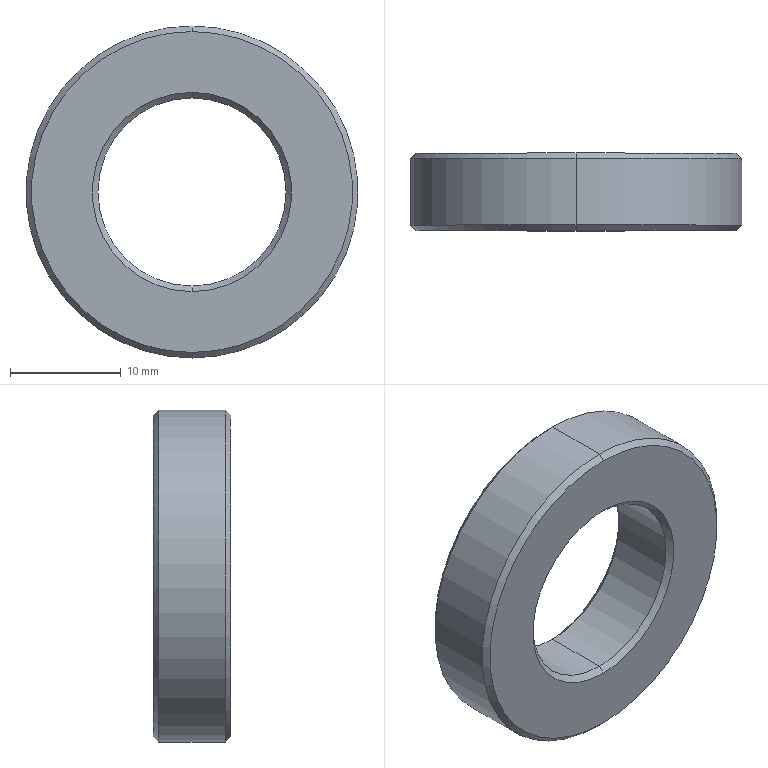Part | STEP file | 6903 ZZ | 1 solid | 14 faces | box 30 x 7 x 30 mm | volume 3322 mm3 | cone 8 | cylinder 4 | plane 2 | commonest cylinder face diameters 17 x2 30 x2
STEP:
#1=CARTESIAN_POINT('',(0.,0.,0.));
#2=DIRECTION('',(0.,0.,1.));
#3=DIRECTION('',(1.,0.,0.));
#4=AXIS2_PLACEMENT_3D('',#1,#2,#3);
#5=CARTESIAN_POINT('',(0.,6.5,8.5));
#6=VERTEX_POINT('',#5);
#7=CARTESIAN_POINT('',(0.,7.,9.));
#8=VERTEX_POINT('',#7);
#9=CARTESIAN_POINT('',(0.,6.5,8.5));
#10=DIRECTION('',(0.,0.7071,0.7071));
#11=VECTOR('',#10,1.);
#12=LINE('',#9,#11);
#13=CARTESIAN_POINT('',(0.,6.5,0.));
#14=DIRECTION('',(0.,1.,0.));
#15=DIRECTION('',(0.,0.,1.));
#16=AXIS2_PLACEMENT_3D('',#13,#14,#15);
#17=CONICAL_SURFACE('',#16,8.5,0.7854);
#18=CARTESIAN_POINT('',(6.283,0.));
#19=DIRECTION('',(0.,1.));
#20=VECTOR('',#19,1.);
#21=LINE('',#18,#20);
#22=(GEOMETRIC_REPRESENTATION_CONTEXT(2)PARAMETRIC_REPRESENTATION_CONTEXT()REPRESENTATION_CONTEXT('',''));
#23=DEFINITIONAL_REPRESENTATION('',(#21),#22);
#24=PCURVE('',#17,#23);
#25=CARTESIAN_POINT('',(0.,6.5,0.));
#26=DIRECTION('',(0.,1.,0.));
#27=DIRECTION('',(0.,0.,1.));
#28=AXIS2_PLACEMENT_3D('',#25,#26,#27);
#29=CONICAL_SURFACE('',#28,8.5,0.7854);
#30=CARTESIAN_POINT('',(0.,0.));
#31=DIRECTION('',(0.,1.));
#32=VECTOR('',#31,1.);
#33=LINE('',#30,#32);
#34=(GEOMETRIC_REPRESENTATION_CONTEXT(2)PARAMETRIC_REPRESENTATION_CONTEXT()REPRESENTATION_CONTEXT('',''));
#35=DEFINITIONAL_REPRESENTATION('',(#33),#34);
#36=PCURVE('',#29,#35);
#37=SURFACE_CURVE('',#12,(#24,#36),.PCURVE_S1.);
#38=EDGE_CURVE('',#6,#8,#37,.T.);
#39=ORIENTED_EDGE('',*,*,#38,.T.);
#40=CARTESIAN_POINT('',(0.,7.,-9.));
#41=VERTEX_POINT('',#40);
#42=CARTESIAN_POINT('',(0.,7.,0.));
#43=DIRECTION('',(0.,-1.,0.));
#44=DIRECTION('',(0.,0.,1.));
#45=AXIS2_PLACEMENT_3D('',#42,#43,#44);
#46=CIRCLE('',#45,9.);
#47=CARTESIAN_POINT('',(6.283,0.5));
#48=DIRECTION('',(-1.,0.));
#49=VECTOR('',#48,1.);
#50=LINE('',#47,#49);
#51=(GEOMETRIC_REPRESENTATION_CONTEXT(2)PARAMETRIC_REPRESENTATION_CONTEXT()REPRESENTATION_CONTEXT('',''));
#52=DEFINITIONAL_REPRESENTATION('',(#50),#51);
#53=PCURVE('',#17,#52);
#54=CARTESIAN_POINT('',(0.,7.,0.));
#55=DIRECTION('',(0.,1.,0.));
#56=DIRECTION('',(0.,0.,1.));
#57=AXIS2_PLACEMENT_3D('',#54,#55,#56);
#58=PLANE('',#57);
#59=CARTESIAN_POINT('',(9.,0.));
#60=CARTESIAN_POINT('',(9.,-15.588));
#61=CARTESIAN_POINT('',(-4.5,-7.794));
#62=CARTESIAN_POINT('',(-18.,0.));
#63=CARTESIAN_POINT('',(-4.5,7.794));
#64=CARTESIAN_POINT('',(9.,15.588));
#65=CARTESIAN_POINT('',(9.,0.));
#66=(BOUNDED_CURVE()B_SPLINE_CURVE(2,(#59,#60,#61,#62,#63,#64,#65),.UNSPECIFIED.,.T.,.F.)B_SPLINE_CURVE_WITH_KNOTS((1,2,2,2,2,1),(-2.094,0.,2.094,4.189,6.283,8.378),.UNSPECIFIED.)CURVE()GEOMETRIC_REPRESENTATION_ITEM()RATIONAL_B_SPLINE_CURVE((1.,0.5,1.,0.5,1.,0.5,1.))REPRESENTATION_ITEM(''));
#67=(GEOMETRIC_REPRESENTATION_CONTEXT(2)PARAMETRIC_REPRESENTATION_CONTEXT()REPRESENTATION_CONTEXT('',''));
#68=DEFINITIONAL_REPRESENTATION('',(#66),#67);
#69=PCURVE('',#58,#68);
#70=SURFACE_CURVE('',#46,(#53,#69),.PCURVE_S1.);
#71=EDGE_CURVE('',#8,#41,#70,.T.);
#72=ORIENTED_EDGE('',*,*,#71,.T.);
#73=CARTESIAN_POINT('',(0.,6.5,-8.5));
#74=VERTEX_POINT('',#73);
#75=CARTESIAN_POINT('',(0.,6.5,-8.5));
#76=DIRECTION('',(0.,0.7071,-0.7071));
#77=VECTOR('',#76,1.);
#78=LINE('',#75,#77);
#79=CARTESIAN_POINT('',(3.142,0.));
#80=DIRECTION('',(0.,1.));
#81=VECTOR('',#80,1.);
#82=LINE('',#79,#81);
#83=(GEOMETRIC_REPRESENTATION_CONTEXT(2)PARAMETRIC_REPRESENTATION_CONTEXT()REPRESENTATION_CONTEXT('',''));
#84=DEFINITIONAL_REPRESENTATION('',(#82),#83);
#85=PCURVE('',#17,#84);
#86=CARTESIAN_POINT('',(3.142,0.));
#87=DIRECTION('',(0.,1.));
#88=VECTOR('',#87,1.);
#89=LINE('',#86,#88);
#90=(GEOMETRIC_REPRESENTATION_CONTEXT(2)PARAMETRIC_REPRESENTATION_CONTEXT()REPRESENTATION_CONTEXT('',''));
#91=DEFINITIONAL_REPRESENTATION('',(#89),#90);
#92=PCURVE('',#29,#91);
#93=SURFACE_CURVE('',#78,(#85,#92),.PCURVE_S1.);
#94=EDGE_CURVE('',#74,#41,#93,.T.);
#95=ORIENTED_EDGE('',*,*,#94,.F.);
#96=CARTESIAN_POINT('',(0.,6.5,0.));
#97=DIRECTION('',(0.,1.,0.));
#98=DIRECTION('',(0.,0.,1.));
#99=AXIS2_PLACEMENT_3D('',#96,#97,#98);
#100=CIRCLE('',#99,8.5);
#101=CARTESIAN_POINT('',(0.,0.));
#102=DIRECTION('',(1.,0.));
#103=VECTOR('',#102,1.);
#104=LINE('',#101,#103);
#105=(GEOMETRIC_REPRESENTATION_CONTEXT(2)PARAMETRIC_REPRESENTATION_CONTEXT()REPRESENTATION_CONTEXT('',''));
#106=DEFINITIONAL_REPRESENTATION('',(#104),#105);
#107=PCURVE('',#17,#106);
#108=CARTESIAN_POINT('',(0.,7.,0.));
#109=DIRECTION('',(0.,-1.,0.));
#110=DIRECTION('',(0.,0.,-1.));
#111=AXIS2_PLACEMENT_3D('',#108,#109,#110);
#112=CYLINDRICAL_SURFACE('',#111,8.5);
#113=CARTESIAN_POINT('',(9.425,0.5));
#114=DIRECTION('',(-1.,0.));
#115=VECTOR('',#114,1.);
#116=LINE('',#113,#115);
#117=(GEOMETRIC_REPRESENTATION_CONTEXT(2)PARAMETRIC_REPRESENTATION_CONTEXT()REPRESENTATION_CONTEXT('',''));
#118=DEFINITIONAL_REPRESENTATION('',(#116),#117);
#119=PCURVE('',#112,#118);
#120=SURFACE_CURVE('',#100,(#107,#119),.PCURVE_S1.);
#121=EDGE_CURVE('',#74,#6,#120,.T.);
#122=ORIENTED_EDGE('',*,*,#121,.T.);
#123=EDGE_LOOP('',(#39,#72,#95,#122));
#124=FACE_BOUND('',#123,.F.);
#125=ADVANCED_FACE('',(#124),#17,.F.);
#126=CARTESIAN_POINT('',(0.,7.,14.5));
#127=VERTEX_POINT('',#126);
#128=CARTESIAN_POINT('',(0.,7.,-14.5));
#129=VERTEX_POINT('',#128);
#130=CARTESIAN_POINT('',(0.,7.,0.));
#131=DIRECTION('',(0.,1.,0.));
#132=DIRECTION('',(0.,0.,1.));
#133=AXIS2_PLACEMENT_3D('',#130,#131,#132);
#134=CIRCLE('',#133,14.5);
#135=CARTESIAN_POINT('',(0.,7.,0.));
#136=DIRECTION('',(0.,-1.,0.));
#137=DIRECTION('',(0.,0.,-1.));
#138=AXIS2_PLACEMENT_3D('',#135,#136,#137);
#139=CONICAL_SURFACE('',#138,14.5,0.7854);
#140=CARTESIAN_POINT('',(3.142,0.));
#141=DIRECTION('',(-1.,0.));
#142=VECTOR('',#141,1.);
#143=LINE('',#140,#142);
#144=(GEOMETRIC_REPRESENTATION_CONTEXT(2)PARAMETRIC_REPRESENTATION_CONTEXT()REPRESENTATION_CONTEXT('',''));
#145=DEFINITIONAL_REPRESENTATION('',(#143),#144);
#146=PCURVE('',#139,#145);
#147=CARTESIAN_POINT('',(0.,0.));
#148=DIRECTION('',(1.,0.));
#149=AXIS2_PLACEMENT_2D('',#147,#148);
#150=CIRCLE('',#149,14.5);
#151=(GEOMETRIC_REPRESENTATION_CONTEXT(2)PARAMETRIC_REPRESENTATION_CONTEXT()REPRESENTATION_CONTEXT('',''));
#152=DEFINITIONAL_REPRESENTATION('',(#150),#151);
#153=PCURVE('',#58,#152);
#154=SURFACE_CURVE('',#134,(#146,#153),.PCURVE_S1.);
#155=EDGE_CURVE('',#127,#129,#154,.T.);
#156=ORIENTED_EDGE('',*,*,#155,.F.);
#157=CARTESIAN_POINT('',(0.,6.5,15.));
#158=VERTEX_POINT('',#157);
#159=CARTESIAN_POINT('',(0.,7.,14.5));
#160=DIRECTION('',(0.,-0.7071,0.7071));
#161=VECTOR('',#160,1.);
#162=LINE('',#159,#161);
#163=CARTESIAN_POINT('',(3.142,0.));
#164=DIRECTION('',(0.,1.));
#165=VECTOR('',#164,1.);
#166=LINE('',#163,#165);
#167=(GEOMETRIC_REPRESENTATION_CONTEXT(2)PARAMETRIC_REPRESENTATION_CONTEXT()REPRESENTATION_CONTEXT('',''));
#168=DEFINITIONAL_REPRESENTATION('',(#166),#167);
#169=PCURVE('',#139,#168);
#170=CARTESIAN_POINT('',(0.,7.,0.));
#171=DIRECTION('',(0.,-1.,0.));
#172=DIRECTION('',(0.,0.,-1.));
#173=AXIS2_PLACEMENT_3D('',#170,#171,#172);
#174=CONICAL_SURFACE('',#173,14.5,0.7854);
#175=CARTESIAN_POINT('',(3.142,0.));
#176=DIRECTION('',(0.,1.));
#177=VECTOR('',#176,1.);
#178=LINE('',#175,#177);
#179=(GEOMETRIC_REPRESENTATION_CONTEXT(2)PARAMETRIC_REPRESENTATION_CONTEXT()REPRESENTATION_CONTEXT('',''));
#180=DEFINITIONAL_REPRESENTATION('',(#178),#179);
#181=PCURVE('',#174,#180);
#182=SURFACE_CURVE('',#162,(#169,#181),.PCURVE_S1.);
#183=EDGE_CURVE('',#127,#158,#182,.T.);
#184=ORIENTED_EDGE('',*,*,#183,.T.);
#185=CARTESIAN_POINT('',(0.,6.5,-15.));
#186=VERTEX_POINT('',#185);
#187=CARTESIAN_POINT('',(0.,6.5,0.));
#188=DIRECTION('',(0.,-1.,0.));
#189=DIRECTION('',(0.,0.,1.));
#190=AXIS2_PLACEMENT_3D('',#187,#188,#189);
#191=CIRCLE('',#190,15.);
#192=CARTESIAN_POINT('',(-3.142,0.5));
#193=DIRECTION('',(1.,0.));
#194=VECTOR('',#193,1.);
#195=LINE('',#192,#194);
#196=(GEOMETRIC_REPRESENTATION_CONTEXT(2)PARAMETRIC_REPRESENTATION_CONTEXT()REPRESENTATION_CONTEXT('',''));
#197=DEFINITIONAL_REPRESENTATION('',(#195),#196);
#198=PCURVE('',#139,#197);
#199=CARTESIAN_POINT('',(0.,7.,0.));
#200=DIRECTION('',(0.,-1.,0.));
#201=DIRECTION('',(0.,0.,-1.));
#202=AXIS2_PLACEMENT_3D('',#199,#200,#201);
#203=CYLINDRICAL_SURFACE('',#202,15.);
#204=CARTESIAN_POINT('',(-3.142,0.5));
#205=DIRECTION('',(1.,0.));
#206=VECTOR('',#205,1.);
#207=LINE('',#204,#206);
#208=(GEOMETRIC_REPRESENTATION_CONTEXT(2)PARAMETRIC_REPRESENTATION_CONTEXT()REPRESENTATION_CONTEXT('',''));
#209=DEFINITIONAL_REPRESENTATION('',(#207),#208);
#210=PCURVE('',#203,#209);
#211=SURFACE_CURVE('',#191,(#198,#210),.PCURVE_S1.);
#212=EDGE_CURVE('',#186,#158,#211,.T.);
#213=ORIENTED_EDGE('',*,*,#212,.F.);
#214=CARTESIAN_POINT('',(0.,7.,-14.5));
#215=DIRECTION('',(0.,-0.7071,-0.7071));
#216=VECTOR('',#215,1.);
#217=LINE('',#214,#216);
#218=CARTESIAN_POINT('',(0.,0.));
#219=DIRECTION('',(0.,1.));
#220=VECTOR('',#219,1.);
#221=LINE('',#218,#220);
#222=(GEOMETRIC_REPRESENTATION_CONTEXT(2)PARAMETRIC_REPRESENTATION_CONTEXT()REPRESENTATION_CONTEXT('',''));
#223=DEFINITIONAL_REPRESENTATION('',(#221),#222);
#224=PCURVE('',#139,#223);
#225=CARTESIAN_POINT('',(6.283,0.));
#226=DIRECTION('',(0.,1.));
#227=VECTOR('',#226,1.);
#228=LINE('',#225,#227);
#229=(GEOMETRIC_REPRESENTATION_CONTEXT(2)PARAMETRIC_REPRESENTATION_CONTEXT()REPRESENTATION_CONTEXT('',''));
#230=DEFINITIONAL_REPRESENTATION('',(#228),#229);
#231=PCURVE('',#174,#230);
#232=SURFACE_CURVE('',#217,(#224,#231),.PCURVE_S1.);
#233=EDGE_CURVE('',#129,#186,#232,.T.);
#234=ORIENTED_EDGE('',*,*,#233,.F.);
#235=EDGE_LOOP('',(#156,#184,#213,#234));
#236=FACE_BOUND('',#235,.T.);
#237=ADVANCED_FACE('',(#236),#139,.T.);
#238=CARTESIAN_POINT('',(0.,0.5,-8.5));
#239=VERTEX_POINT('',#238);
#240=CARTESIAN_POINT('',(0.,0.,-9.));
#241=VERTEX_POINT('',#240);
#242=CARTESIAN_POINT('',(0.,0.,-9.));
#243=DIRECTION('',(0.,-0.7071,-0.7071));
#244=VECTOR('',#243,1.);
#245=LINE('',#242,#244);
#246=CARTESIAN_POINT('',(0.,0.,0.));
#247=DIRECTION('',(0.,-1.,0.));
#248=DIRECTION('',(0.,0.,-1.));
#249=AXIS2_PLACEMENT_3D('',#246,#247,#248);
#250=CONICAL_SURFACE('',#249,9.,0.7854);
#251=CARTESIAN_POINT('',(6.283,0.));
#252=DIRECTION('',(0.,1.));
#253=VECTOR('',#252,1.);
#254=LINE('',#251,#253);
#255=(GEOMETRIC_REPRESENTATION_CONTEXT(2)PARAMETRIC_REPRESENTATION_CONTEXT()REPRESENTATION_CONTEXT('',''));
#256=DEFINITIONAL_REPRESENTATION('',(#254),#255);
#257=PCURVE('',#250,#256);
#258=CARTESIAN_POINT('',(0.,0.,0.));
#259=DIRECTION('',(0.,-1.,0.));
#260=DIRECTION('',(0.,0.,-1.));
#261=AXIS2_PLACEMENT_3D('',#258,#259,#260);
#262=CONICAL_SURFACE('',#261,9.,0.7854);
#263=CARTESIAN_POINT('',(0.,0.));
#264=DIRECTION('',(0.,1.));
#265=VECTOR('',#264,1.);
#266=LINE('',#263,#265);
#267=(GEOMETRIC_REPRESENTATION_CONTEXT(2)PARAMETRIC_REPRESENTATION_CONTEXT()REPRESENTATION_CONTEXT('',''));
#268=DEFINITIONAL_REPRESENTATION('',(#266),#267);
#269=PCURVE('',#262,#268);
#270=SURFACE_CURVE('',#245,(#257,#269),.PCURVE_S1.);
#271=EDGE_CURVE('',#239,#241,#270,.T.);
#272=ORIENTED_EDGE('',*,*,#271,.T.);
#273=CARTESIAN_POINT('',(0.,0.,9.));
#274=VERTEX_POINT('',#273);
#275=CARTESIAN_POINT('',(0.,0.,0.));
#276=DIRECTION('',(0.,1.,0.));
#277=DIRECTION('',(0.,0.,1.));
#278=AXIS2_PLACEMENT_3D('',#275,#276,#277);
#279=CIRCLE('',#278,9.);
#280=CARTESIAN_POINT('',(9.425,0.));
#281=DIRECTION('',(-1.,0.));
#282=VECTOR('',#281,1.);
#283=LINE('',#280,#282);
#284=(GEOMETRIC_REPRESENTATION_CONTEXT(2)PARAMETRIC_REPRESENTATION_CONTEXT()REPRESENTATION_CONTEXT('',''));
#285=DEFINITIONAL_REPRESENTATION('',(#283),#284);
#286=PCURVE('',#250,#285);
#287=CARTESIAN_POINT('',(0.,0.,0.));
#288=DIRECTION('',(0.,1.,0.));
#289=DIRECTION('',(0.,0.,1.));
#290=AXIS2_PLACEMENT_3D('',#287,#288,#289);
#291=PLANE('',#290);
#292=CARTESIAN_POINT('',(0.,0.));
#293=DIRECTION('',(1.,0.));
#294=AXIS2_PLACEMENT_2D('',#292,#293);
#295=CIRCLE('',#294,9.);
#296=(GEOMETRIC_REPRESENTATION_CONTEXT(2)PARAMETRIC_REPRESENTATION_CONTEXT()REPRESENTATION_CONTEXT('',''));
#297=DEFINITIONAL_REPRESENTATION('',(#295),#296);
#298=PCURVE('',#291,#297);
#299=SURFACE_CURVE('',#279,(#286,#298),.PCURVE_S1.);
#300=EDGE_CURVE('',#241,#274,#299,.T.);
#301=ORIENTED_EDGE('',*,*,#300,.T.);
#302=CARTESIAN_POINT('',(0.,0.5,8.5));
#303=VERTEX_POINT('',#302);
#304=CARTESIAN_POINT('',(0.,0.,9.));
#305=DIRECTION('',(0.,-0.7071,0.7071));
#306=VECTOR('',#305,1.);
#307=LINE('',#304,#306);
#308=CARTESIAN_POINT('',(3.142,0.));
#309=DIRECTION('',(0.,1.));
#310=VECTOR('',#309,1.);
#311=LINE('',#308,#310);
#312=(GEOMETRIC_REPRESENTATION_CONTEXT(2)PARAMETRIC_REPRESENTATION_CONTEXT()REPRESENTATION_CONTEXT('',''));
#313=DEFINITIONAL_REPRESENTATION('',(#311),#312);
#314=PCURVE('',#250,#313);
#315=CARTESIAN_POINT('',(3.142,0.));
#316=DIRECTION('',(0.,1.));
#317=VECTOR('',#316,1.);
#318=LINE('',#315,#317);
#319=(GEOMETRIC_REPRESENTATION_CONTEXT(2)PARAMETRIC_REPRESENTATION_CONTEXT()REPRESENTATION_CONTEXT('',''));
#320=DEFINITIONAL_REPRESENTATION('',(#318),#319);
#321=PCURVE('',#262,#320);
#322=SURFACE_CURVE('',#307,(#314,#321),.PCURVE_S1.);
#323=EDGE_CURVE('',#303,#274,#322,.T.);
#324=ORIENTED_EDGE('',*,*,#323,.F.);
#325=CARTESIAN_POINT('',(0.,0.5,0.));
#326=DIRECTION('',(0.,-1.,0.));
#327=DIRECTION('',(0.,0.,1.));
#328=AXIS2_PLACEMENT_3D('',#325,#326,#327);
#329=CIRCLE('',#328,8.5);
#330=CARTESIAN_POINT('',(3.142,-0.5));
#331=DIRECTION('',(1.,0.));
#332=VECTOR('',#331,1.);
#333=LINE('',#330,#332);
#334=(GEOMETRIC_REPRESENTATION_CONTEXT(2)PARAMETRIC_REPRESENTATION_CONTEXT()REPRESENTATION_CONTEXT('',''));
#335=DEFINITIONAL_REPRESENTATION('',(#333),#334);
#336=PCURVE('',#250,#335);
#337=CARTESIAN_POINT('',(3.142,6.5));
#338=DIRECTION('',(1.,0.));
#339=VECTOR('',#338,1.);
#340=LINE('',#337,#339);
#341=(GEOMETRIC_REPRESENTATION_CONTEXT(2)PARAMETRIC_REPRESENTATION_CONTEXT()REPRESENTATION_CONTEXT('',''));
#342=DEFINITIONAL_REPRESENTATION('',(#340),#341);
#343=PCURVE('',#112,#342);
#344=SURFACE_CURVE('',#329,(#336,#343),.PCURVE_S1.);
#345=EDGE_CURVE('',#303,#239,#344,.T.);
#346=ORIENTED_EDGE('',*,*,#345,.T.);
#347=EDGE_LOOP('',(#272,#301,#324,#346));
#348=FACE_BOUND('',#347,.F.);
#349=ADVANCED_FACE('',(#348),#250,.F.);
#350=CARTESIAN_POINT('',(0.,0.,-14.5));
#351=VERTEX_POINT('',#350);
#352=CARTESIAN_POINT('',(0.,0.,14.5));
#353=VERTEX_POINT('',#352);
#354=CARTESIAN_POINT('',(0.,0.,0.));
#355=DIRECTION('',(0.,-1.,0.));
#356=DIRECTION('',(0.,0.,1.));
#357=AXIS2_PLACEMENT_3D('',#354,#355,#356);
#358=CIRCLE('',#357,14.5);
#359=CARTESIAN_POINT('',(0.,0.5,0.));
#360=DIRECTION('',(0.,1.,0.));
#361=DIRECTION('',(0.,0.,1.));
#362=AXIS2_PLACEMENT_3D('',#359,#360,#361);
#363=CONICAL_SURFACE('',#362,15.,0.7854);
#364=CARTESIAN_POINT('',(6.283,-0.5));
#365=DIRECTION('',(-1.,0.));
#366=VECTOR('',#365,1.);
#367=LINE('',#364,#366);
#368=(GEOMETRIC_REPRESENTATION_CONTEXT(2)PARAMETRIC_REPRESENTATION_CONTEXT()REPRESENTATION_CONTEXT('',''));
#369=DEFINITIONAL_REPRESENTATION('',(#367),#368);
#370=PCURVE('',#363,#369);
#371=CARTESIAN_POINT('',(14.5,0.));
#372=CARTESIAN_POINT('',(14.5,-25.115));
#373=CARTESIAN_POINT('',(-7.25,-12.557));
#374=CARTESIAN_POINT('',(-29.,0.));
#375=CARTESIAN_POINT('',(-7.25,12.557));
#376=CARTESIAN_POINT('',(14.5,25.115));
#377=CARTESIAN_POINT('',(14.5,0.));
#378=(BOUNDED_CURVE()B_SPLINE_CURVE(2,(#371,#372,#373,#374,#375,#376,#377),.UNSPECIFIED.,.T.,.F.)B_SPLINE_CURVE_WITH_KNOTS((1,2,2,2,2,1),(-2.094,0.,2.094,4.189,6.283,8.378),.UNSPECIFIED.)CURVE()GEOMETRIC_REPRESENTATION_ITEM()RATIONAL_B_SPLINE_CURVE((1.,0.5,1.,0.5,1.,0.5,1.))REPRESENTATION_ITEM(''));
#379=(GEOMETRIC_REPRESENTATION_CONTEXT(2)PARAMETRIC_REPRESENTATION_CONTEXT()REPRESENTATION_CONTEXT('',''));
#380=DEFINITIONAL_REPRESENTATION('',(#378),#379);
#381=PCURVE('',#291,#380);
#382=SURFACE_CURVE('',#358,(#370,#381),.PCURVE_S1.);
#383=EDGE_CURVE('',#351,#353,#382,.T.);
#384=ORIENTED_EDGE('',*,*,#383,.F.);
#385=CARTESIAN_POINT('',(0.,0.5,-15.));
#386=VERTEX_POINT('',#385);
#387=CARTESIAN_POINT('',(0.,0.5,-15.));
#388=DIRECTION('',(0.,0.7071,-0.7071));
#389=VECTOR('',#388,1.);
#390=LINE('',#387,#389);
#391=CARTESIAN_POINT('',(3.142,0.));
#392=DIRECTION('',(0.,1.));
#393=VECTOR('',#392,1.);
#394=LINE('',#391,#393);
#395=(GEOMETRIC_REPRESENTATION_CONTEXT(2)PARAMETRIC_REPRESENTATION_CONTEXT()REPRESENTATION_CONTEXT('',''));
#396=DEFINITIONAL_REPRESENTATION('',(#394),#395);
#397=PCURVE('',#363,#396);
#398=CARTESIAN_POINT('',(0.,0.5,0.));
#399=DIRECTION('',(0.,1.,0.));
#400=DIRECTION('',(0.,0.,1.));
#401=AXIS2_PLACEMENT_3D('',#398,#399,#400);
#402=CONICAL_SURFACE('',#401,15.,0.7854);
#403=CARTESIAN_POINT('',(3.142,0.));
#404=DIRECTION('',(0.,1.));
#405=VECTOR('',#404,1.);
#406=LINE('',#403,#405);
#407=(GEOMETRIC_REPRESENTATION_CONTEXT(2)PARAMETRIC_REPRESENTATION_CONTEXT()REPRESENTATION_CONTEXT('',''));
#408=DEFINITIONAL_REPRESENTATION('',(#406),#407);
#409=PCURVE('',#402,#408);
#410=SURFACE_CURVE('',#390,(#397,#409),.PCURVE_S1.);
#411=EDGE_CURVE('',#351,#386,#410,.T.);
#412=ORIENTED_EDGE('',*,*,#411,.T.);
#413=CARTESIAN_POINT('',(0.,0.5,15.));
#414=VERTEX_POINT('',#413);
#415=CARTESIAN_POINT('',(0.,0.5,0.));
#416=DIRECTION('',(0.,1.,0.));
#417=DIRECTION('',(0.,0.,1.));
#418=AXIS2_PLACEMENT_3D('',#415,#416,#417);
#419=CIRCLE('',#418,15.);
#420=CARTESIAN_POINT('',(0.,0.));
#421=DIRECTION('',(1.,0.));
#422=VECTOR('',#421,1.);
#423=LINE('',#420,#422);
#424=(GEOMETRIC_REPRESENTATION_CONTEXT(2)PARAMETRIC_REPRESENTATION_CONTEXT()REPRESENTATION_CONTEXT('',''));
#425=DEFINITIONAL_REPRESENTATION('',(#423),#424);
#426=PCURVE('',#363,#425);
#427=CARTESIAN_POINT('',(3.142,6.5));
#428=DIRECTION('',(-1.,0.));
#429=VECTOR('',#428,1.);
#430=LINE('',#427,#429);
#431=(GEOMETRIC_REPRESENTATION_CONTEXT(2)PARAMETRIC_REPRESENTATION_CONTEXT()REPRESENTATION_CONTEXT('',''));
#432=DEFINITIONAL_REPRESENTATION('',(#430),#431);
#433=PCURVE('',#203,#432);
#434=SURFACE_CURVE('',#419,(#426,#433),.PCURVE_S1.);
#435=EDGE_CURVE('',#414,#386,#434,.T.);
#436=ORIENTED_EDGE('',*,*,#435,.F.);
#437=CARTESIAN_POINT('',(0.,0.5,15.));
#438=DIRECTION('',(0.,0.7071,0.7071));
#439=VECTOR('',#438,1.);
#440=LINE('',#437,#439);
#441=CARTESIAN_POINT('',(0.,0.));
#442=DIRECTION('',(0.,1.));
#443=VECTOR('',#442,1.);
#444=LINE('',#441,#443);
#445=(GEOMETRIC_REPRESENTATION_CONTEXT(2)PARAMETRIC_REPRESENTATION_CONTEXT()REPRESENTATION_CONTEXT('',''));
#446=DEFINITIONAL_REPRESENTATION('',(#444),#445);
#447=PCURVE('',#363,#446);
#448=CARTESIAN_POINT('',(6.283,0.));
#449=DIRECTION('',(0.,1.));
#450=VECTOR('',#449,1.);
#451=LINE('',#448,#450);
#452=(GEOMETRIC_REPRESENTATION_CONTEXT(2)PARAMETRIC_REPRESENTATION_CONTEXT()REPRESENTATION_CONTEXT('',''));
#453=DEFINITIONAL_REPRESENTATION('',(#451),#452);
#454=PCURVE('',#402,#453);
#455=SURFACE_CURVE('',#440,(#447,#454),.PCURVE_S1.);
#456=EDGE_CURVE('',#353,#414,#455,.T.);
#457=ORIENTED_EDGE('',*,*,#456,.F.);
#458=EDGE_LOOP('',(#384,#412,#436,#457));
#459=FACE_BOUND('',#458,.T.);
#460=ADVANCED_FACE('',(#459),#363,.T.);
#461=CARTESIAN_POINT('',(0.,7.,-8.5));
#462=DIRECTION('',(0.,-1.,0.));
#463=VECTOR('',#462,1.);
#464=LINE('',#461,#463);
#465=CARTESIAN_POINT('',(6.283,0.));
#466=DIRECTION('',(0.,1.));
#467=VECTOR('',#466,1.);
#468=LINE('',#465,#467);
#469=(GEOMETRIC_REPRESENTATION_CONTEXT(2)PARAMETRIC_REPRESENTATION_CONTEXT()REPRESENTATION_CONTEXT('',''));
#470=DEFINITIONAL_REPRESENTATION('',(#468),#469);
#471=PCURVE('',#112,#470);
#472=CARTESIAN_POINT('',(0.,7.,0.));
#473=DIRECTION('',(0.,-1.,0.));
#474=DIRECTION('',(0.,0.,-1.));
#475=AXIS2_PLACEMENT_3D('',#472,#473,#474);
#476=CYLINDRICAL_SURFACE('',#475,8.5);
#477=CARTESIAN_POINT('',(0.,0.));
#478=DIRECTION('',(0.,1.));
#479=VECTOR('',#478,1.);
#480=LINE('',#477,#479);
#481=(GEOMETRIC_REPRESENTATION_CONTEXT(2)PARAMETRIC_REPRESENTATION_CONTEXT()REPRESENTATION_CONTEXT('',''));
#482=DEFINITIONAL_REPRESENTATION('',(#480),#481);
#483=PCURVE('',#476,#482);
#484=SURFACE_CURVE('',#464,(#471,#483),.PCURVE_S1.);
#485=EDGE_CURVE('',#74,#239,#484,.T.);
#486=ORIENTED_EDGE('',*,*,#485,.T.);
#487=ORIENTED_EDGE('',*,*,#345,.F.);
#488=CARTESIAN_POINT('',(0.,7.,8.5));
#489=DIRECTION('',(0.,-1.,0.));
#490=VECTOR('',#489,1.);
#491=LINE('',#488,#490);
#492=CARTESIAN_POINT('',(3.142,0.));
#493=DIRECTION('',(0.,1.));
#494=VECTOR('',#493,1.);
#495=LINE('',#492,#494);
#496=(GEOMETRIC_REPRESENTATION_CONTEXT(2)PARAMETRIC_REPRESENTATION_CONTEXT()REPRESENTATION_CONTEXT('',''));
#497=DEFINITIONAL_REPRESENTATION('',(#495),#496);
#498=PCURVE('',#112,#497);
#499=CARTESIAN_POINT('',(3.142,0.));
#500=DIRECTION('',(0.,1.));
#501=VECTOR('',#500,1.);
#502=LINE('',#499,#501);
#503=(GEOMETRIC_REPRESENTATION_CONTEXT(2)PARAMETRIC_REPRESENTATION_CONTEXT()REPRESENTATION_CONTEXT('',''));
#504=DEFINITIONAL_REPRESENTATION('',(#502),#503);
#505=PCURVE('',#476,#504);
#506=SURFACE_CURVE('',#491,(#498,#505),.PCURVE_S1.);
#507=EDGE_CURVE('',#6,#303,#506,.T.);
#508=ORIENTED_EDGE('',*,*,#507,.F.);
#509=ORIENTED_EDGE('',*,*,#121,.F.);
#510=EDGE_LOOP('',(#486,#487,#508,#509));
#511=FACE_BOUND('',#510,.F.);
#512=ADVANCED_FACE('',(#511),#112,.F.);
#513=ORIENTED_EDGE('',*,*,#212,.T.);
#514=CARTESIAN_POINT('',(0.,7.,15.));
#515=DIRECTION('',(0.,-1.,0.));
#516=VECTOR('',#515,1.);
#517=LINE('',#514,#516);
#518=CARTESIAN_POINT('',(3.142,0.));
#519=DIRECTION('',(0.,1.));
#520=VECTOR('',#519,1.);
#521=LINE('',#518,#520);
#522=(GEOMETRIC_REPRESENTATION_CONTEXT(2)PARAMETRIC_REPRESENTATION_CONTEXT()REPRESENTATION_CONTEXT('',''));
#523=DEFINITIONAL_REPRESENTATION('',(#521),#522);
#524=PCURVE('',#203,#523);
#525=CARTESIAN_POINT('',(0.,7.,0.));
#526=DIRECTION('',(0.,-1.,0.));
#527=DIRECTION('',(0.,0.,-1.));
#528=AXIS2_PLACEMENT_3D('',#525,#526,#527);
#529=CYLINDRICAL_SURFACE('',#528,15.);
#530=CARTESIAN_POINT('',(3.142,0.));
#531=DIRECTION('',(0.,1.));
#532=VECTOR('',#531,1.);
#533=LINE('',#530,#532);
#534=(GEOMETRIC_REPRESENTATION_CONTEXT(2)PARAMETRIC_REPRESENTATION_CONTEXT()REPRESENTATION_CONTEXT('',''));
#535=DEFINITIONAL_REPRESENTATION('',(#533),#534);
#536=PCURVE('',#529,#535);
#537=SURFACE_CURVE('',#517,(#524,#536),.PCURVE_S1.);
#538=EDGE_CURVE('',#158,#414,#537,.T.);
#539=ORIENTED_EDGE('',*,*,#538,.T.);
#540=ORIENTED_EDGE('',*,*,#435,.T.);
#541=CARTESIAN_POINT('',(0.,7.,-15.));
#542=DIRECTION('',(0.,-1.,0.));
#543=VECTOR('',#542,1.);
#544=LINE('',#541,#543);
#545=CARTESIAN_POINT('',(0.,0.));
#546=DIRECTION('',(0.,1.));
#547=VECTOR('',#546,1.);
#548=LINE('',#545,#547);
#549=(GEOMETRIC_REPRESENTATION_CONTEXT(2)PARAMETRIC_REPRESENTATION_CONTEXT()REPRESENTATION_CONTEXT('',''));
#550=DEFINITIONAL_REPRESENTATION('',(#548),#549);
#551=PCURVE('',#203,#550);
#552=CARTESIAN_POINT('',(6.283,0.));
#553=DIRECTION('',(0.,1.));
#554=VECTOR('',#553,1.);
#555=LINE('',#552,#554);
#556=(GEOMETRIC_REPRESENTATION_CONTEXT(2)PARAMETRIC_REPRESENTATION_CONTEXT()REPRESENTATION_CONTEXT('',''));
#557=DEFINITIONAL_REPRESENTATION('',(#555),#556);
#558=PCURVE('',#529,#557);
#559=SURFACE_CURVE('',#544,(#551,#558),.PCURVE_S1.);
#560=EDGE_CURVE('',#186,#386,#559,.T.);
#561=ORIENTED_EDGE('',*,*,#560,.F.);
#562=EDGE_LOOP('',(#513,#539,#540,#561));
#563=FACE_BOUND('',#562,.T.);
#564=ADVANCED_FACE('',(#563),#203,.T.);
#565=CARTESIAN_POINT('',(0.,7.,0.));
#566=DIRECTION('',(0.,1.,0.));
#567=DIRECTION('',(0.,0.,1.));
#568=AXIS2_PLACEMENT_3D('',#565,#566,#567);
#569=CIRCLE('',#568,14.5);
#570=CARTESIAN_POINT('',(0.,0.));
#571=DIRECTION('',(1.,0.));
#572=AXIS2_PLACEMENT_2D('',#570,#571);
#573=CIRCLE('',#572,14.5);
#574=(GEOMETRIC_REPRESENTATION_CONTEXT(2)PARAMETRIC_REPRESENTATION_CONTEXT()REPRESENTATION_CONTEXT('',''));
#575=DEFINITIONAL_REPRESENTATION('',(#573),#574);
#576=PCURVE('',#58,#575);
#577=CARTESIAN_POINT('',(9.425,0.));
#578=DIRECTION('',(-1.,0.));
#579=VECTOR('',#578,1.);
#580=LINE('',#577,#579);
#581=(GEOMETRIC_REPRESENTATION_CONTEXT(2)PARAMETRIC_REPRESENTATION_CONTEXT()REPRESENTATION_CONTEXT('',''));
#582=DEFINITIONAL_REPRESENTATION('',(#580),#581);
#583=PCURVE('',#174,#582);
#584=SURFACE_CURVE('',#569,(#576,#583),.PCURVE_S1.);
#585=EDGE_CURVE('',#129,#127,#584,.T.);
#586=ORIENTED_EDGE('',*,*,#585,.T.);
#587=ORIENTED_EDGE('',*,*,#155,.T.);
#588=EDGE_LOOP('',(#586,#587));
#589=FACE_BOUND('',#588,.T.);
#590=ORIENTED_EDGE('',*,*,#71,.T.);
#591=CARTESIAN_POINT('',(0.,7.,0.));
#592=DIRECTION('',(0.,-1.,0.));
#593=DIRECTION('',(0.,0.,1.));
#594=AXIS2_PLACEMENT_3D('',#591,#592,#593);
#595=CIRCLE('',#594,9.);
#596=CARTESIAN_POINT('',(9.,0.));
#597=CARTESIAN_POINT('',(9.,-15.588));
#598=CARTESIAN_POINT('',(-4.5,-7.794));
#599=CARTESIAN_POINT('',(-18.,0.));
#600=CARTESIAN_POINT('',(-4.5,7.794));
#601=CARTESIAN_POINT('',(9.,15.588));
#602=CARTESIAN_POINT('',(9.,0.));
#603=(BOUNDED_CURVE()B_SPLINE_CURVE(2,(#596,#597,#598,#599,#600,#601,#602),.UNSPECIFIED.,.T.,.F.)B_SPLINE_CURVE_WITH_KNOTS((1,2,2,2,2,1),(-2.094,0.,2.094,4.189,6.283,8.378),.UNSPECIFIED.)CURVE()GEOMETRIC_REPRESENTATION_ITEM()RATIONAL_B_SPLINE_CURVE((1.,0.5,1.,0.5,1.,0.5,1.))REPRESENTATION_ITEM(''));
#604=(GEOMETRIC_REPRESENTATION_CONTEXT(2)PARAMETRIC_REPRESENTATION_CONTEXT()REPRESENTATION_CONTEXT('',''));
#605=DEFINITIONAL_REPRESENTATION('',(#603),#604);
#606=PCURVE('',#58,#605);
#607=CARTESIAN_POINT('',(6.283,0.5));
#608=DIRECTION('',(-1.,0.));
#609=VECTOR('',#608,1.);
#610=LINE('',#607,#609);
#611=(GEOMETRIC_REPRESENTATION_CONTEXT(2)PARAMETRIC_REPRESENTATION_CONTEXT()REPRESENTATION_CONTEXT('',''));
#612=DEFINITIONAL_REPRESENTATION('',(#610),#611);
#613=PCURVE('',#29,#612);
#614=SURFACE_CURVE('',#595,(#606,#613),.PCURVE_S1.);
#615=EDGE_CURVE('',#41,#8,#614,.T.);
#616=ORIENTED_EDGE('',*,*,#615,.T.);
#617=EDGE_LOOP('',(#590,#616));
#618=FACE_BOUND('',#617,.T.);
#619=ADVANCED_FACE('',(#589,#618),#58,.T.);
#620=CARTESIAN_POINT('',(0.,0.,0.));
#621=DIRECTION('',(0.,-1.,0.));
#622=DIRECTION('',(0.,0.,1.));
#623=AXIS2_PLACEMENT_3D('',#620,#621,#622);
#624=CIRCLE('',#623,14.5);
#625=CARTESIAN_POINT('',(14.5,0.));
#626=CARTESIAN_POINT('',(14.5,-25.115));
#627=CARTESIAN_POINT('',(-7.25,-12.557));
#628=CARTESIAN_POINT('',(-29.,0.));
#629=CARTESIAN_POINT('',(-7.25,12.557));
#630=CARTESIAN_POINT('',(14.5,25.115));
#631=CARTESIAN_POINT('',(14.5,0.));
#632=(BOUNDED_CURVE()B_SPLINE_CURVE(2,(#625,#626,#627,#628,#629,#630,#631),.UNSPECIFIED.,.T.,.F.)B_SPLINE_CURVE_WITH_KNOTS((1,2,2,2,2,1),(-2.094,0.,2.094,4.189,6.283,8.378),.UNSPECIFIED.)CURVE()GEOMETRIC_REPRESENTATION_ITEM()RATIONAL_B_SPLINE_CURVE((1.,0.5,1.,0.5,1.,0.5,1.))REPRESENTATION_ITEM(''));
#633=(GEOMETRIC_REPRESENTATION_CONTEXT(2)PARAMETRIC_REPRESENTATION_CONTEXT()REPRESENTATION_CONTEXT('',''));
#634=DEFINITIONAL_REPRESENTATION('',(#632),#633);
#635=PCURVE('',#291,#634);
#636=CARTESIAN_POINT('',(6.283,-0.5));
#637=DIRECTION('',(-1.,0.));
#638=VECTOR('',#637,1.);
#639=LINE('',#636,#638);
#640=(GEOMETRIC_REPRESENTATION_CONTEXT(2)PARAMETRIC_REPRESENTATION_CONTEXT()REPRESENTATION_CONTEXT('',''));
#641=DEFINITIONAL_REPRESENTATION('',(#639),#640);
#642=PCURVE('',#402,#641);
#643=SURFACE_CURVE('',#624,(#635,#642),.PCURVE_S1.);
#644=EDGE_CURVE('',#353,#351,#643,.T.);
#645=ORIENTED_EDGE('',*,*,#644,.T.);
#646=ORIENTED_EDGE('',*,*,#383,.T.);
#647=EDGE_LOOP('',(#645,#646));
#648=FACE_BOUND('',#647,.T.);
#649=ORIENTED_EDGE('',*,*,#300,.T.);
#650=CARTESIAN_POINT('',(0.,0.,0.));
#651=DIRECTION('',(0.,1.,0.));
#652=DIRECTION('',(0.,0.,1.));
#653=AXIS2_PLACEMENT_3D('',#650,#651,#652);
#654=CIRCLE('',#653,9.);
#655=CARTESIAN_POINT('',(0.,0.));
#656=DIRECTION('',(1.,0.));
#657=AXIS2_PLACEMENT_2D('',#655,#656);
#658=CIRCLE('',#657,9.);
#659=(GEOMETRIC_REPRESENTATION_CONTEXT(2)PARAMETRIC_REPRESENTATION_CONTEXT()REPRESENTATION_CONTEXT('',''));
#660=DEFINITIONAL_REPRESENTATION('',(#658),#659);
#661=PCURVE('',#291,#660);
#662=CARTESIAN_POINT('',(3.142,0.));
#663=DIRECTION('',(-1.,0.));
#664=VECTOR('',#663,1.);
#665=LINE('',#662,#664);
#666=(GEOMETRIC_REPRESENTATION_CONTEXT(2)PARAMETRIC_REPRESENTATION_CONTEXT()REPRESENTATION_CONTEXT('',''));
#667=DEFINITIONAL_REPRESENTATION('',(#665),#666);
#668=PCURVE('',#262,#667);
#669=SURFACE_CURVE('',#654,(#661,#668),.PCURVE_S1.);
#670=EDGE_CURVE('',#274,#241,#669,.T.);
#671=ORIENTED_EDGE('',*,*,#670,.T.);
#672=EDGE_LOOP('',(#649,#671));
#673=FACE_BOUND('',#672,.T.);
#674=ADVANCED_FACE('',(#648,#673),#291,.F.);
#675=ORIENTED_EDGE('',*,*,#538,.F.);
#676=CARTESIAN_POINT('',(0.,6.5,0.));
#677=DIRECTION('',(0.,-1.,0.));
#678=DIRECTION('',(0.,0.,1.));
#679=AXIS2_PLACEMENT_3D('',#676,#677,#678);
#680=CIRCLE('',#679,15.);
#681=CARTESIAN_POINT('',(3.142,0.5));
#682=DIRECTION('',(1.,0.));
#683=VECTOR('',#682,1.);
#684=LINE('',#681,#683);
#685=(GEOMETRIC_REPRESENTATION_CONTEXT(2)PARAMETRIC_REPRESENTATION_CONTEXT()REPRESENTATION_CONTEXT('',''));
#686=DEFINITIONAL_REPRESENTATION('',(#684),#685);
#687=PCURVE('',#529,#686);
#688=CARTESIAN_POINT('',(3.142,0.5));
#689=DIRECTION('',(1.,0.));
#690=VECTOR('',#689,1.);
#691=LINE('',#688,#690);
#692=(GEOMETRIC_REPRESENTATION_CONTEXT(2)PARAMETRIC_REPRESENTATION_CONTEXT()REPRESENTATION_CONTEXT('',''));
#693=DEFINITIONAL_REPRESENTATION('',(#691),#692);
#694=PCURVE('',#174,#693);
#695=SURFACE_CURVE('',#680,(#687,#694),.PCURVE_S1.);
#696=EDGE_CURVE('',#158,#186,#695,.T.);
#697=ORIENTED_EDGE('',*,*,#696,.T.);
#698=ORIENTED_EDGE('',*,*,#560,.T.);
#699=CARTESIAN_POINT('',(0.,0.5,0.));
#700=DIRECTION('',(0.,1.,0.));
#701=DIRECTION('',(0.,0.,1.));
#702=AXIS2_PLACEMENT_3D('',#699,#700,#701);
#703=CIRCLE('',#702,15.);
#704=CARTESIAN_POINT('',(9.425,6.5));
#705=DIRECTION('',(-1.,0.));
#706=VECTOR('',#705,1.);
#707=LINE('',#704,#706);
#708=(GEOMETRIC_REPRESENTATION_CONTEXT(2)PARAMETRIC_REPRESENTATION_CONTEXT()REPRESENTATION_CONTEXT('',''));
#709=DEFINITIONAL_REPRESENTATION('',(#707),#708);
#710=PCURVE('',#529,#709);
#711=CARTESIAN_POINT('',(0.,0.));
#712=DIRECTION('',(1.,0.));
#713=VECTOR('',#712,1.);
#714=LINE('',#711,#713);
#715=(GEOMETRIC_REPRESENTATION_CONTEXT(2)PARAMETRIC_REPRESENTATION_CONTEXT()REPRESENTATION_CONTEXT('',''));
#716=DEFINITIONAL_REPRESENTATION('',(#714),#715);
#717=PCURVE('',#402,#716);
#718=SURFACE_CURVE('',#703,(#710,#717),.PCURVE_S1.);
#719=EDGE_CURVE('',#386,#414,#718,.T.);
#720=ORIENTED_EDGE('',*,*,#719,.T.);
#721=EDGE_LOOP('',(#675,#697,#698,#720));
#722=FACE_BOUND('',#721,.T.);
#723=ADVANCED_FACE('',(#722),#529,.T.);
#724=CARTESIAN_POINT('',(0.,0.5,0.));
#725=DIRECTION('',(0.,-1.,0.));
#726=DIRECTION('',(0.,0.,1.));
#727=AXIS2_PLACEMENT_3D('',#724,#725,#726);
#728=CIRCLE('',#727,8.5);
#729=CARTESIAN_POINT('',(-3.142,6.5));
#730=DIRECTION('',(1.,0.));
#731=VECTOR('',#730,1.);
#732=LINE('',#729,#731);
#733=(GEOMETRIC_REPRESENTATION_CONTEXT(2)PARAMETRIC_REPRESENTATION_CONTEXT()REPRESENTATION_CONTEXT('',''));
#734=DEFINITIONAL_REPRESENTATION('',(#732),#733);
#735=PCURVE('',#476,#734);
#736=CARTESIAN_POINT('',(-3.142,-0.5));
#737=DIRECTION('',(1.,0.));
#738=VECTOR('',#737,1.);
#739=LINE('',#736,#738);
#740=(GEOMETRIC_REPRESENTATION_CONTEXT(2)PARAMETRIC_REPRESENTATION_CONTEXT()REPRESENTATION_CONTEXT('',''));
#741=DEFINITIONAL_REPRESENTATION('',(#739),#740);
#742=PCURVE('',#262,#741);
#743=SURFACE_CURVE('',#728,(#735,#742),.PCURVE_S1.);
#744=EDGE_CURVE('',#239,#303,#743,.T.);
#745=ORIENTED_EDGE('',*,*,#744,.F.);
#746=ORIENTED_EDGE('',*,*,#485,.F.);
#747=CARTESIAN_POINT('',(0.,6.5,0.));
#748=DIRECTION('',(0.,1.,0.));
#749=DIRECTION('',(0.,0.,1.));
#750=AXIS2_PLACEMENT_3D('',#747,#748,#749);
#751=CIRCLE('',#750,8.5);
#752=CARTESIAN_POINT('',(3.142,0.5));
#753=DIRECTION('',(-1.,0.));
#754=VECTOR('',#753,1.);
#755=LINE('',#752,#754);
#756=(GEOMETRIC_REPRESENTATION_CONTEXT(2)PARAMETRIC_REPRESENTATION_CONTEXT()REPRESENTATION_CONTEXT('',''));
#757=DEFINITIONAL_REPRESENTATION('',(#755),#756);
#758=PCURVE('',#476,#757);
#759=CARTESIAN_POINT('',(0.,0.));
#760=DIRECTION('',(1.,0.));
#761=VECTOR('',#760,1.);
#762=LINE('',#759,#761);
#763=(GEOMETRIC_REPRESENTATION_CONTEXT(2)PARAMETRIC_REPRESENTATION_CONTEXT()REPRESENTATION_CONTEXT('',''));
#764=DEFINITIONAL_REPRESENTATION('',(#762),#763);
#765=PCURVE('',#29,#764);
#766=SURFACE_CURVE('',#751,(#758,#765),.PCURVE_S1.);
#767=EDGE_CURVE('',#6,#74,#766,.T.);
#768=ORIENTED_EDGE('',*,*,#767,.F.);
#769=ORIENTED_EDGE('',*,*,#507,.T.);
#770=EDGE_LOOP('',(#745,#746,#768,#769));
#771=FACE_BOUND('',#770,.F.);
#772=ADVANCED_FACE('',(#771),#476,.F.);
#773=ORIENTED_EDGE('',*,*,#411,.F.);
#774=ORIENTED_EDGE('',*,*,#644,.F.);
#775=ORIENTED_EDGE('',*,*,#456,.T.);
#776=ORIENTED_EDGE('',*,*,#719,.F.);
#777=EDGE_LOOP('',(#773,#774,#775,#776));
#778=FACE_BOUND('',#777,.T.);
#779=ADVANCED_FACE('',(#778),#402,.T.);
#780=ORIENTED_EDGE('',*,*,#670,.T.);
#781=ORIENTED_EDGE('',*,*,#271,.F.);
#782=ORIENTED_EDGE('',*,*,#744,.T.);
#783=ORIENTED_EDGE('',*,*,#323,.T.);
#784=EDGE_LOOP('',(#780,#781,#782,#783));
#785=FACE_BOUND('',#784,.F.);
#786=ADVANCED_FACE('',(#785),#262,.F.);
#787=ORIENTED_EDGE('',*,*,#183,.F.);
#788=ORIENTED_EDGE('',*,*,#585,.F.);
#789=ORIENTED_EDGE('',*,*,#233,.T.);
#790=ORIENTED_EDGE('',*,*,#696,.F.);
#791=EDGE_LOOP('',(#787,#788,#789,#790));
#792=FACE_BOUND('',#791,.T.);
#793=ADVANCED_FACE('',(#792),#174,.T.);
#794=ORIENTED_EDGE('',*,*,#615,.T.);
#795=ORIENTED_EDGE('',*,*,#38,.F.);
#796=ORIENTED_EDGE('',*,*,#767,.T.);
#797=ORIENTED_EDGE('',*,*,#94,.T.);
#798=EDGE_LOOP('',(#794,#795,#796,#797));
#799=FACE_BOUND('',#798,.F.);
#800=ADVANCED_FACE('',(#799),#29,.F.);
#801=CLOSED_SHELL('',(#125,#237,#349,#460,#512,#564,#619,#674,#723,#772,#779,#786,#793,#800));
#802=MANIFOLD_SOLID_BREP('',#801);
#803=(LENGTH_UNIT()NAMED_UNIT(*)SI_UNIT(.MILLI.,.METRE.));
#804=UNCERTAINTY_MEASURE_WITH_UNIT(LENGTH_MEASURE(0.0000001),#803,'','');
#805=(NAMED_UNIT(*)PLANE_ANGLE_UNIT()SI_UNIT($,.RADIAN.));
#806=(NAMED_UNIT(*)SI_UNIT($,.STERADIAN.)SOLID_ANGLE_UNIT());
#807=(GEOMETRIC_REPRESENTATION_CONTEXT(3)GLOBAL_UNCERTAINTY_ASSIGNED_CONTEXT((#804))GLOBAL_UNIT_ASSIGNED_CONTEXT((#803,#805,#806))REPRESENTATION_CONTEXT('',''));
#808=ADVANCED_BREP_SHAPE_REPRESENTATION('',(#4,#802),#807);